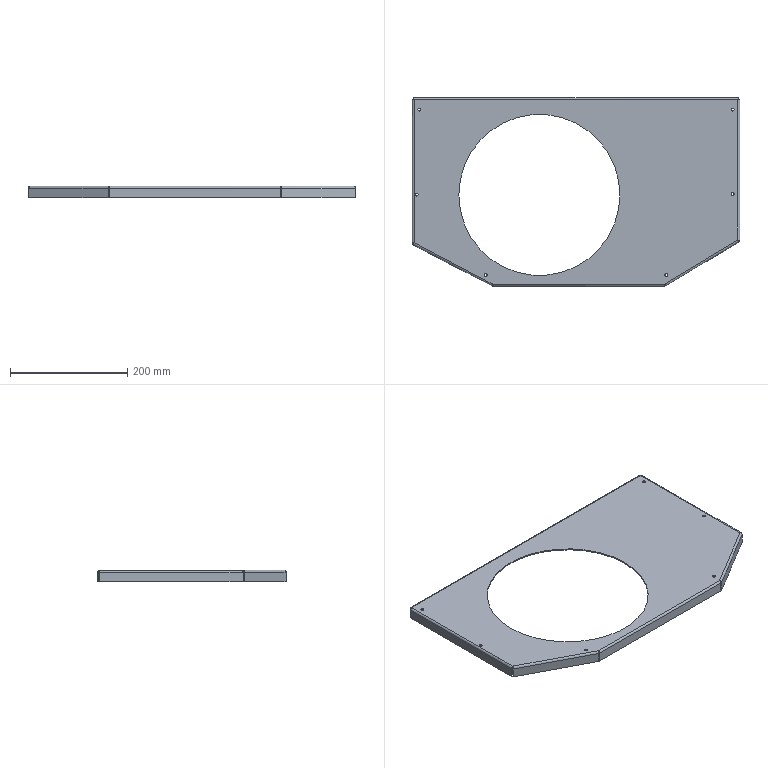Part | STEP file | Housing cover plate SGN-2-31-03 | 1 solid | 70 faces | box 560 x 322 x 20 mm | volume 277072 mm3 | plane 32 | cylinder 26 | spline 12 | commonest cylinder face diameters 5 x12 3 x6 7 x6 275 x2